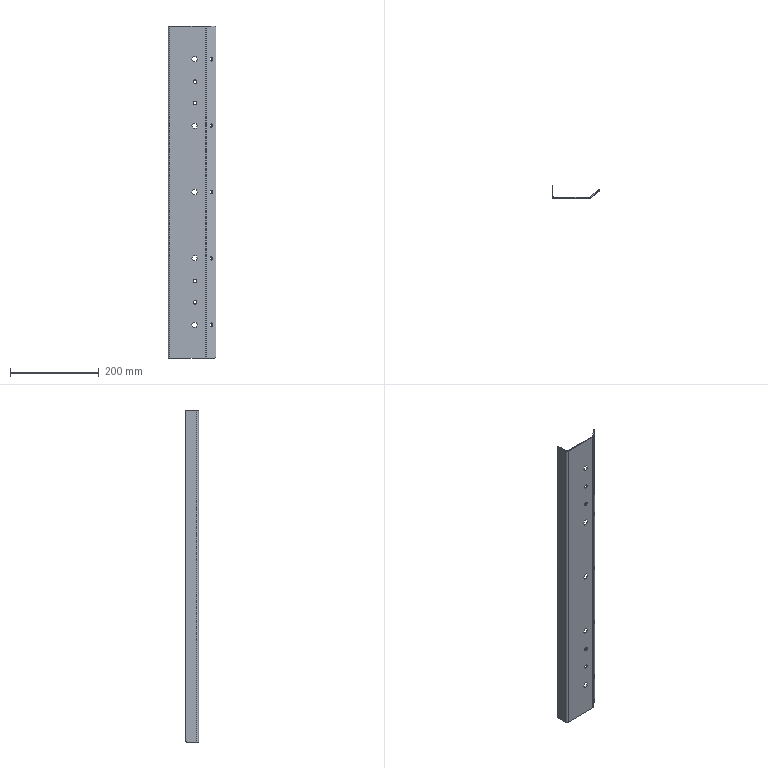Part | STEP file | Side panel wer5 BeforeLift N7 | 1 solid | 65 faces | box 107.981 x 30 x 750 mm | volume 209231 mm3 | plane 48 | cylinder 17 | commonest cylinder face diameters 8.2 x9 6 x4 4 x2 8 x2